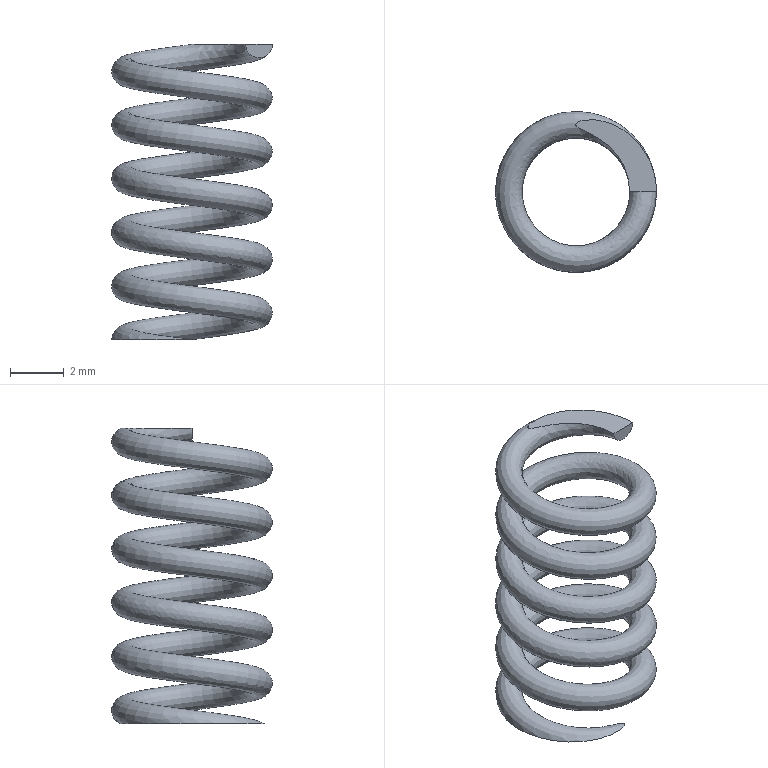Part | STEP file | gslz 2016.10.28-6_id510_x_t | 1 solid | 4 faces | box 5.996 x 5.994 x 11 mm | volume 66.438 mm3 | plane 3 | spline 1